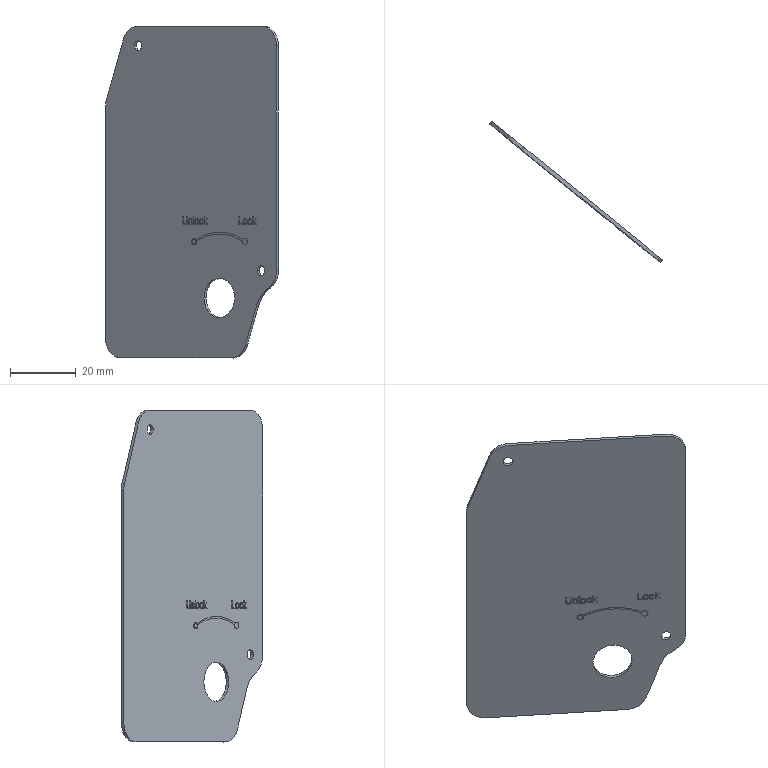Part | SolidWorks | features BaseBody 1 | 1 solid | 950 faces | box 52.612 x 43.048 x 101 mm | volume 6311 mm3 | plane 927 | cylinder 23 | commonest cylinder face diameters 12 x8 2 x6 3 x4 1.455 x2 20 x1 39 x1